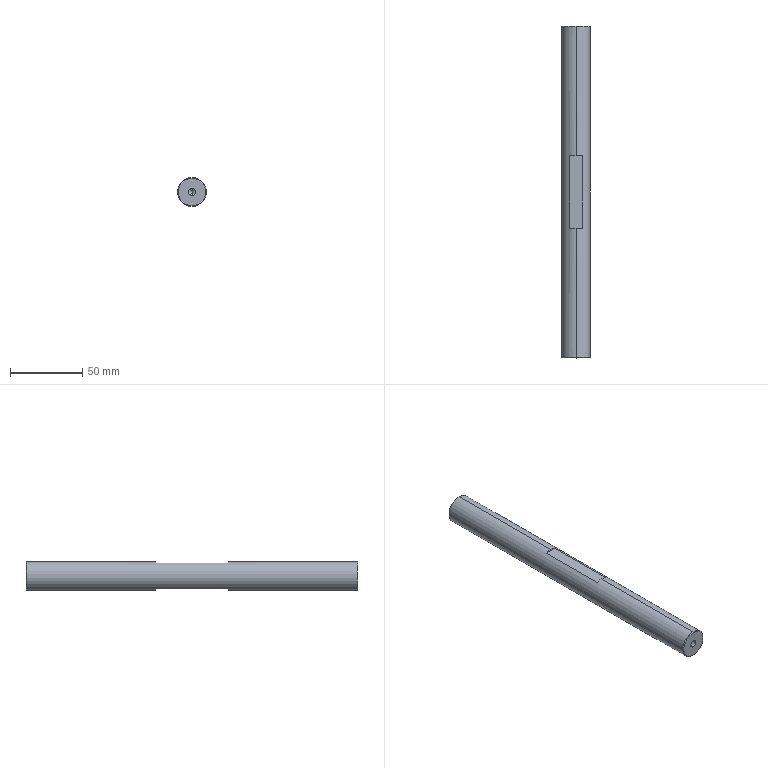Part | STEP file | PN_0026 | 1 solid | 25 faces | box 20 x 230 x 20 mm | volume 70863 mm3 | plane 9 | cone 8 | cylinder 8 | commonest cylinder face diameters 5 x4 6 x2 20 x2